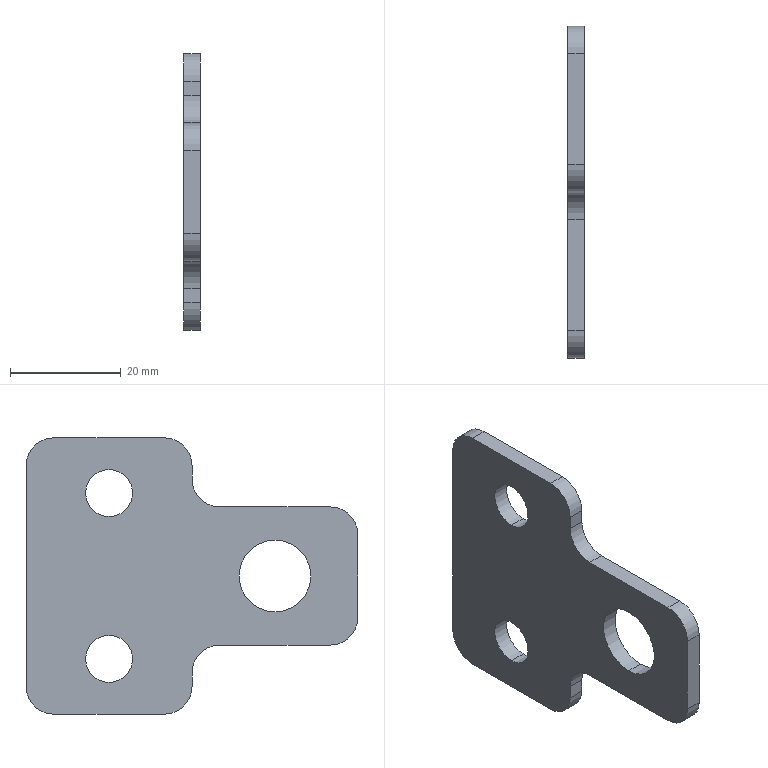Part | SolidWorks | features HoleWzd 2, Fillet 1, FlatPattern 1, ICE 1, SMBaseFlange 1, SheetMetal 1 | 1 solid | 24 faces | box 3 x 60 x 50 mm | volume 5947 mm3 | cylinder 14 | plane 10 | commonest cylinder face diameters 10 x8 8.5 x4 13 x2
STEP:
#1=CARTESIAN_POINT('',(-3.,-15.,6.5));
#2=VERTEX_POINT('',#1);
#3=CARTESIAN_POINT('',(-3.,-15.,-6.5));
#4=VERTEX_POINT('',#3);
#5=CARTESIAN_POINT('',(-3.,-15.,0.));
#6=DIRECTION('',(1.,0.,0.));
#7=DIRECTION('',(0.,0.,-1.));
#8=AXIS2_PLACEMENT_3D('',#5,#6,#7);
#9=CIRCLE('',#8,6.5);
#10=EDGE_CURVE('',#2,#4,#9,.T.);
#11=ORIENTED_EDGE('',*,*,#10,.F.);
#12=CARTESIAN_POINT('',(0.,-15.,6.5));
#13=VERTEX_POINT('',#12);
#14=CARTESIAN_POINT('',(0.,-15.,6.5));
#15=DIRECTION('',(1.,0.,0.));
#16=VECTOR('',#15,1000.);
#17=LINE('',#14,#16);
#18=EDGE_CURVE('',#2,#13,#17,.T.);
#19=ORIENTED_EDGE('',*,*,#18,.T.);
#20=CARTESIAN_POINT('',(0.,-15.,-6.5));
#21=VERTEX_POINT('',#20);
#22=CARTESIAN_POINT('',(0.,-15.,0.));
#23=DIRECTION('',(1.,0.,0.));
#24=DIRECTION('',(0.,0.,-1.));
#25=AXIS2_PLACEMENT_3D('',#22,#23,#24);
#26=CIRCLE('',#25,6.5);
#27=EDGE_CURVE('',#13,#21,#26,.T.);
#28=ORIENTED_EDGE('',*,*,#27,.T.);
#29=CARTESIAN_POINT('',(0.,-15.,-6.5));
#30=DIRECTION('',(1.,0.,0.));
#31=VECTOR('',#30,1000.);
#32=LINE('',#29,#31);
#33=EDGE_CURVE('',#4,#21,#32,.T.);
#34=ORIENTED_EDGE('',*,*,#33,.F.);
#35=EDGE_LOOP('',(#11,#19,#28,#34));
#36=FACE_OUTER_BOUND('',#35,.T.);
#37=CARTESIAN_POINT('',(0.,-15.,0.));
#38=DIRECTION('',(1.,0.,0.));
#39=DIRECTION('',(0.,0.,-1.));
#40=AXIS2_PLACEMENT_3D('',#37,#38,#39);
#41=CYLINDRICAL_SURFACE('',#40,6.5);
#42=ADVANCED_FACE('',(#36),#41,.F.);
#43=CARTESIAN_POINT('',(-3.,15.,19.25));
#44=VERTEX_POINT('',#43);
#45=CARTESIAN_POINT('',(-3.,15.,10.75));
#46=VERTEX_POINT('',#45);
#47=CARTESIAN_POINT('',(-3.,15.,15.));
#48=DIRECTION('',(1.,0.,0.));
#49=DIRECTION('',(0.,0.,-1.));
#50=AXIS2_PLACEMENT_3D('',#47,#48,#49);
#51=CIRCLE('',#50,4.25);
#52=EDGE_CURVE('',#44,#46,#51,.T.);
#53=ORIENTED_EDGE('',*,*,#52,.F.);
#54=CARTESIAN_POINT('',(0.,15.,19.25));
#55=VERTEX_POINT('',#54);
#56=CARTESIAN_POINT('',(0.,15.,19.25));
#57=DIRECTION('',(1.,0.,0.));
#58=VECTOR('',#57,1000.);
#59=LINE('',#56,#58);
#60=EDGE_CURVE('',#44,#55,#59,.T.);
#61=ORIENTED_EDGE('',*,*,#60,.T.);
#62=CARTESIAN_POINT('',(0.,15.,10.75));
#63=VERTEX_POINT('',#62);
#64=CARTESIAN_POINT('',(0.,15.,15.));
#65=DIRECTION('',(1.,0.,0.));
#66=DIRECTION('',(0.,0.,-1.));
#67=AXIS2_PLACEMENT_3D('',#64,#65,#66);
#68=CIRCLE('',#67,4.25);
#69=EDGE_CURVE('',#55,#63,#68,.T.);
#70=ORIENTED_EDGE('',*,*,#69,.T.);
#71=CARTESIAN_POINT('',(0.,15.,10.75));
#72=DIRECTION('',(1.,0.,0.));
#73=VECTOR('',#72,1000.);
#74=LINE('',#71,#73);
#75=EDGE_CURVE('',#46,#63,#74,.T.);
#76=ORIENTED_EDGE('',*,*,#75,.F.);
#77=EDGE_LOOP('',(#53,#61,#70,#76));
#78=FACE_OUTER_BOUND('',#77,.T.);
#79=CARTESIAN_POINT('',(0.,15.,15.));
#80=DIRECTION('',(1.,0.,0.));
#81=DIRECTION('',(0.,0.,-1.));
#82=AXIS2_PLACEMENT_3D('',#79,#80,#81);
#83=CYLINDRICAL_SURFACE('',#82,4.25);
#84=ADVANCED_FACE('',(#78),#83,.F.);
#85=CARTESIAN_POINT('',(-3.,15.,-10.75));
#86=VERTEX_POINT('',#85);
#87=CARTESIAN_POINT('',(-3.,15.,-19.25));
#88=VERTEX_POINT('',#87);
#89=CARTESIAN_POINT('',(-3.,15.,-15.));
#90=DIRECTION('',(1.,0.,0.));
#91=DIRECTION('',(0.,0.,-1.));
#92=AXIS2_PLACEMENT_3D('',#89,#90,#91);
#93=CIRCLE('',#92,4.25);
#94=EDGE_CURVE('',#86,#88,#93,.T.);
#95=ORIENTED_EDGE('',*,*,#94,.F.);
#96=CARTESIAN_POINT('',(0.,15.,-10.75));
#97=VERTEX_POINT('',#96);
#98=CARTESIAN_POINT('',(0.,15.,-10.75));
#99=DIRECTION('',(1.,0.,0.));
#100=VECTOR('',#99,1000.);
#101=LINE('',#98,#100);
#102=EDGE_CURVE('',#86,#97,#101,.T.);
#103=ORIENTED_EDGE('',*,*,#102,.T.);
#104=CARTESIAN_POINT('',(0.,15.,-19.25));
#105=VERTEX_POINT('',#104);
#106=CARTESIAN_POINT('',(0.,15.,-15.));
#107=DIRECTION('',(1.,0.,0.));
#108=DIRECTION('',(0.,0.,-1.));
#109=AXIS2_PLACEMENT_3D('',#106,#107,#108);
#110=CIRCLE('',#109,4.25);
#111=EDGE_CURVE('',#97,#105,#110,.T.);
#112=ORIENTED_EDGE('',*,*,#111,.T.);
#113=CARTESIAN_POINT('',(0.,15.,-19.25));
#114=DIRECTION('',(1.,0.,0.));
#115=VECTOR('',#114,1000.);
#116=LINE('',#113,#115);
#117=EDGE_CURVE('',#88,#105,#116,.T.);
#118=ORIENTED_EDGE('',*,*,#117,.F.);
#119=EDGE_LOOP('',(#95,#103,#112,#118));
#120=FACE_OUTER_BOUND('',#119,.T.);
#121=CARTESIAN_POINT('',(0.,15.,-15.));
#122=DIRECTION('',(1.,0.,0.));
#123=DIRECTION('',(0.,0.,-1.));
#124=AXIS2_PLACEMENT_3D('',#121,#122,#123);
#125=CYLINDRICAL_SURFACE('',#124,4.25);
#126=ADVANCED_FACE('',(#120),#125,.F.);
#127=CARTESIAN_POINT('',(0.,5.,-25.));
#128=VERTEX_POINT('',#127);
#129=CARTESIAN_POINT('',(0.,25.,-25.));
#130=VERTEX_POINT('',#129);
#131=CARTESIAN_POINT('',(0.,30.,-25.));
#132=DIRECTION('',(0.,1.,0.));
#133=VECTOR('',#132,1000.);
#134=LINE('',#131,#133);
#135=EDGE_CURVE('',#128,#130,#134,.T.);
#136=ORIENTED_EDGE('',*,*,#135,.F.);
#137=CARTESIAN_POINT('',(-3.,5.,-25.));
#138=VERTEX_POINT('',#137);
#139=CARTESIAN_POINT('',(-3.,5.,-25.));
#140=DIRECTION('',(-1.,0.,0.));
#141=VECTOR('',#140,1000.);
#142=LINE('',#139,#141);
#143=EDGE_CURVE('',#128,#138,#142,.T.);
#144=ORIENTED_EDGE('',*,*,#143,.T.);
#145=CARTESIAN_POINT('',(-3.,25.,-25.));
#146=VERTEX_POINT('',#145);
#147=CARTESIAN_POINT('',(-3.,30.,-25.));
#148=DIRECTION('',(0.,1.,0.));
#149=VECTOR('',#148,1000.);
#150=LINE('',#147,#149);
#151=EDGE_CURVE('',#138,#146,#150,.T.);
#152=ORIENTED_EDGE('',*,*,#151,.T.);
#153=CARTESIAN_POINT('',(-3.,25.,-25.));
#154=DIRECTION('',(1.,0.,0.));
#155=VECTOR('',#154,1000.);
#156=LINE('',#153,#155);
#157=EDGE_CURVE('',#146,#130,#156,.T.);
#158=ORIENTED_EDGE('',*,*,#157,.T.);
#159=EDGE_LOOP('',(#136,#144,#152,#158));
#160=FACE_OUTER_BOUND('',#159,.T.);
#161=CARTESIAN_POINT('',(-3.,30.,-25.));
#162=DIRECTION('',(0.,0.,-1.));
#163=DIRECTION('',(0.,1.,0.));
#164=AXIS2_PLACEMENT_3D('',#161,#162,#163);
#165=PLANE('',#164);
#166=ADVANCED_FACE('',(#160),#165,.T.);
#167=CARTESIAN_POINT('',(0.,-30.,7.5));
#168=VERTEX_POINT('',#167);
#169=CARTESIAN_POINT('',(0.,-30.,-7.5));
#170=VERTEX_POINT('',#169);
#171=CARTESIAN_POINT('',(0.,-30.,25.));
#172=DIRECTION('',(0.,0.,-1.));
#173=VECTOR('',#172,1000.);
#174=LINE('',#171,#173);
#175=EDGE_CURVE('',#168,#170,#174,.T.);
#176=ORIENTED_EDGE('',*,*,#175,.F.);
#177=CARTESIAN_POINT('',(-3.,-30.,7.5));
#178=VERTEX_POINT('',#177);
#179=CARTESIAN_POINT('',(-3.,-30.,7.5));
#180=DIRECTION('',(-1.,0.,0.));
#181=VECTOR('',#180,1000.);
#182=LINE('',#179,#181);
#183=EDGE_CURVE('',#168,#178,#182,.T.);
#184=ORIENTED_EDGE('',*,*,#183,.T.);
#185=CARTESIAN_POINT('',(-3.,-30.,-7.5));
#186=VERTEX_POINT('',#185);
#187=CARTESIAN_POINT('',(-3.,-30.,25.));
#188=DIRECTION('',(0.,0.,-1.));
#189=VECTOR('',#188,1000.);
#190=LINE('',#187,#189);
#191=EDGE_CURVE('',#178,#186,#190,.T.);
#192=ORIENTED_EDGE('',*,*,#191,.T.);
#193=CARTESIAN_POINT('',(0.,-30.,-7.5));
#194=DIRECTION('',(1.,0.,0.));
#195=VECTOR('',#194,1000.);
#196=LINE('',#193,#195);
#197=EDGE_CURVE('',#186,#170,#196,.T.);
#198=ORIENTED_EDGE('',*,*,#197,.T.);
#199=EDGE_LOOP('',(#176,#184,#192,#198));
#200=FACE_OUTER_BOUND('',#199,.T.);
#201=CARTESIAN_POINT('',(-3.,-30.,25.));
#202=DIRECTION('',(0.,-1.,0.));
#203=DIRECTION('',(0.,0.,-1.));
#204=AXIS2_PLACEMENT_3D('',#201,#202,#203);
#205=PLANE('',#204);
#206=ADVANCED_FACE('',(#200),#205,.T.);
#207=CARTESIAN_POINT('',(-3.,25.,25.));
#208=VERTEX_POINT('',#207);
#209=CARTESIAN_POINT('',(-3.,5.,25.));
#210=VERTEX_POINT('',#209);
#211=CARTESIAN_POINT('',(-3.,30.,25.));
#212=DIRECTION('',(0.,-1.,0.));
#213=VECTOR('',#212,1000.);
#214=LINE('',#211,#213);
#215=EDGE_CURVE('',#208,#210,#214,.T.);
#216=ORIENTED_EDGE('',*,*,#215,.T.);
#217=CARTESIAN_POINT('',(0.,5.,25.));
#218=VERTEX_POINT('',#217);
#219=CARTESIAN_POINT('',(0.,5.,25.));
#220=DIRECTION('',(1.,0.,0.));
#221=VECTOR('',#220,1000.);
#222=LINE('',#219,#221);
#223=EDGE_CURVE('',#210,#218,#222,.T.);
#224=ORIENTED_EDGE('',*,*,#223,.T.);
#225=CARTESIAN_POINT('',(0.,25.,25.));
#226=VERTEX_POINT('',#225);
#227=CARTESIAN_POINT('',(0.,30.,25.));
#228=DIRECTION('',(0.,-1.,0.));
#229=VECTOR('',#228,1000.);
#230=LINE('',#227,#229);
#231=EDGE_CURVE('',#226,#218,#230,.T.);
#232=ORIENTED_EDGE('',*,*,#231,.F.);
#233=CARTESIAN_POINT('',(-3.,25.,25.));
#234=DIRECTION('',(-1.,0.,0.));
#235=VECTOR('',#234,1000.);
#236=LINE('',#233,#235);
#237=EDGE_CURVE('',#226,#208,#236,.T.);
#238=ORIENTED_EDGE('',*,*,#237,.T.);
#239=EDGE_LOOP('',(#216,#224,#232,#238));
#240=FACE_OUTER_BOUND('',#239,.T.);
#241=CARTESIAN_POINT('',(-3.,30.,25.));
#242=DIRECTION('',(0.,0.,1.));
#243=DIRECTION('',(0.,-1.,0.));
#244=AXIS2_PLACEMENT_3D('',#241,#242,#243);
#245=PLANE('',#244);
#246=ADVANCED_FACE('',(#240),#245,.T.);
#247=CARTESIAN_POINT('',(0.,30.,-20.));
#248=VERTEX_POINT('',#247);
#249=CARTESIAN_POINT('',(0.,30.,20.));
#250=VERTEX_POINT('',#249);
#251=CARTESIAN_POINT('',(0.,30.,25.));
#252=DIRECTION('',(0.,0.,1.));
#253=VECTOR('',#252,1000.);
#254=LINE('',#251,#253);
#255=EDGE_CURVE('',#248,#250,#254,.T.);
#256=ORIENTED_EDGE('',*,*,#255,.F.);
#257=CARTESIAN_POINT('',(-3.,30.,-20.));
#258=VERTEX_POINT('',#257);
#259=CARTESIAN_POINT('',(-3.,30.,-20.));
#260=DIRECTION('',(-1.,0.,0.));
#261=VECTOR('',#260,1000.);
#262=LINE('',#259,#261);
#263=EDGE_CURVE('',#248,#258,#262,.T.);
#264=ORIENTED_EDGE('',*,*,#263,.T.);
#265=CARTESIAN_POINT('',(-3.,30.,20.));
#266=VERTEX_POINT('',#265);
#267=CARTESIAN_POINT('',(-3.,30.,25.));
#268=DIRECTION('',(0.,0.,1.));
#269=VECTOR('',#268,1000.);
#270=LINE('',#267,#269);
#271=EDGE_CURVE('',#258,#266,#270,.T.);
#272=ORIENTED_EDGE('',*,*,#271,.T.);
#273=CARTESIAN_POINT('',(-3.,30.,20.));
#274=DIRECTION('',(1.,0.,0.));
#275=VECTOR('',#274,1000.);
#276=LINE('',#273,#275);
#277=EDGE_CURVE('',#266,#250,#276,.T.);
#278=ORIENTED_EDGE('',*,*,#277,.T.);
#279=EDGE_LOOP('',(#256,#264,#272,#278));
#280=FACE_OUTER_BOUND('',#279,.T.);
#281=CARTESIAN_POINT('',(-3.,30.,25.));
#282=DIRECTION('',(0.,1.,0.));
#283=DIRECTION('',(0.,0.,1.));
#284=AXIS2_PLACEMENT_3D('',#281,#282,#283);
#285=PLANE('',#284);
#286=ADVANCED_FACE('',(#280),#285,.T.);
#287=CARTESIAN_POINT('',(-3.,-15.,0.));
#288=DIRECTION('',(1.,0.,0.));
#289=DIRECTION('',(0.,0.,-1.));
#290=AXIS2_PLACEMENT_3D('',#287,#288,#289);
#291=CIRCLE('',#290,6.5);
#292=EDGE_CURVE('',#4,#2,#291,.T.);
#293=ORIENTED_EDGE('',*,*,#292,.T.);
#294=ORIENTED_EDGE('',*,*,#10,.T.);
#295=EDGE_LOOP('',(#293,#294));
#296=FACE_BOUND('',#295,.T.);
#297=CARTESIAN_POINT('',(-3.,15.,15.));
#298=DIRECTION('',(1.,0.,0.));
#299=DIRECTION('',(0.,0.,-1.));
#300=AXIS2_PLACEMENT_3D('',#297,#298,#299);
#301=CIRCLE('',#300,4.25);
#302=EDGE_CURVE('',#46,#44,#301,.T.);
#303=ORIENTED_EDGE('',*,*,#302,.T.);
#304=ORIENTED_EDGE('',*,*,#52,.T.);
#305=EDGE_LOOP('',(#303,#304));
#306=FACE_BOUND('',#305,.T.);
#307=CARTESIAN_POINT('',(-3.,15.,-15.));
#308=DIRECTION('',(1.,0.,0.));
#309=DIRECTION('',(0.,0.,-1.));
#310=AXIS2_PLACEMENT_3D('',#307,#308,#309);
#311=CIRCLE('',#310,4.25);
#312=EDGE_CURVE('',#88,#86,#311,.T.);
#313=ORIENTED_EDGE('',*,*,#312,.T.);
#314=ORIENTED_EDGE('',*,*,#94,.T.);
#315=EDGE_LOOP('',(#313,#314));
#316=FACE_BOUND('',#315,.T.);
#317=ORIENTED_EDGE('',*,*,#191,.F.);
#318=CARTESIAN_POINT('',(-3.,-25.,12.5));
#319=VERTEX_POINT('',#318);
#320=CARTESIAN_POINT('',(-3.,-25.,7.5));
#321=DIRECTION('',(-1.,0.,0.));
#322=DIRECTION('',(0.,0.,-1.));
#323=AXIS2_PLACEMENT_3D('',#320,#321,#322);
#324=CIRCLE('',#323,5.);
#325=EDGE_CURVE('',#178,#319,#324,.T.);
#326=ORIENTED_EDGE('',*,*,#325,.T.);
#327=CARTESIAN_POINT('',(-3.,-5.,12.5));
#328=VERTEX_POINT('',#327);
#329=CARTESIAN_POINT('',(-3.,-30.,12.5));
#330=DIRECTION('',(0.,1.,0.));
#331=VECTOR('',#330,1000.);
#332=LINE('',#329,#331);
#333=EDGE_CURVE('',#319,#328,#332,.T.);
#334=ORIENTED_EDGE('',*,*,#333,.T.);
#335=CARTESIAN_POINT('',(-3.,0.,17.5));
#336=VERTEX_POINT('',#335);
#337=CARTESIAN_POINT('',(-3.,-5.,17.5));
#338=DIRECTION('',(1.,0.,0.));
#339=DIRECTION('',(0.,0.,-1.));
#340=AXIS2_PLACEMENT_3D('',#337,#338,#339);
#341=CIRCLE('',#340,5.);
#342=EDGE_CURVE('',#328,#336,#341,.T.);
#343=ORIENTED_EDGE('',*,*,#342,.T.);
#344=CARTESIAN_POINT('',(-3.,0.,20.));
#345=VERTEX_POINT('',#344);
#346=CARTESIAN_POINT('',(-3.,0.,25.));
#347=DIRECTION('',(0.,0.,1.));
#348=VECTOR('',#347,1000.);
#349=LINE('',#346,#348);
#350=EDGE_CURVE('',#336,#345,#349,.T.);
#351=ORIENTED_EDGE('',*,*,#350,.T.);
#352=CARTESIAN_POINT('',(-3.,5.,20.));
#353=DIRECTION('',(-1.,0.,0.));
#354=DIRECTION('',(0.,0.,-1.));
#355=AXIS2_PLACEMENT_3D('',#352,#353,#354);
#356=CIRCLE('',#355,5.);
#357=EDGE_CURVE('',#345,#210,#356,.T.);
#358=ORIENTED_EDGE('',*,*,#357,.T.);
#359=ORIENTED_EDGE('',*,*,#215,.F.);
#360=CARTESIAN_POINT('',(-3.,25.,20.));
#361=DIRECTION('',(-1.,0.,0.));
#362=DIRECTION('',(0.,0.,-1.));
#363=AXIS2_PLACEMENT_3D('',#360,#361,#362);
#364=CIRCLE('',#363,5.);
#365=EDGE_CURVE('',#208,#266,#364,.T.);
#366=ORIENTED_EDGE('',*,*,#365,.T.);
#367=ORIENTED_EDGE('',*,*,#271,.F.);
#368=CARTESIAN_POINT('',(-3.,25.,-20.));
#369=DIRECTION('',(-1.,0.,0.));
#370=DIRECTION('',(0.,0.,-1.));
#371=AXIS2_PLACEMENT_3D('',#368,#369,#370);
#372=CIRCLE('',#371,5.);
#373=EDGE_CURVE('',#258,#146,#372,.T.);
#374=ORIENTED_EDGE('',*,*,#373,.T.);
#375=ORIENTED_EDGE('',*,*,#151,.F.);
#376=CARTESIAN_POINT('',(-3.,0.,-20.));
#377=VERTEX_POINT('',#376);
#378=CARTESIAN_POINT('',(-3.,5.,-20.));
#379=DIRECTION('',(-1.,0.,0.));
#380=DIRECTION('',(0.,0.,-1.));
#381=AXIS2_PLACEMENT_3D('',#378,#379,#380);
#382=CIRCLE('',#381,5.);
#383=EDGE_CURVE('',#138,#377,#382,.T.);
#384=ORIENTED_EDGE('',*,*,#383,.T.);
#385=CARTESIAN_POINT('',(-3.,0.,-17.5));
#386=VERTEX_POINT('',#385);
#387=CARTESIAN_POINT('',(-3.,0.,-25.));
#388=DIRECTION('',(0.,0.,1.));
#389=VECTOR('',#388,1000.);
#390=LINE('',#387,#389);
#391=EDGE_CURVE('',#377,#386,#390,.T.);
#392=ORIENTED_EDGE('',*,*,#391,.T.);
#393=CARTESIAN_POINT('',(-3.,-5.,-12.5));
#394=VERTEX_POINT('',#393);
#395=CARTESIAN_POINT('',(-3.,-5.,-17.5));
#396=DIRECTION('',(1.,0.,0.));
#397=DIRECTION('',(0.,0.,-1.));
#398=AXIS2_PLACEMENT_3D('',#395,#396,#397);
#399=CIRCLE('',#398,5.);
#400=EDGE_CURVE('',#386,#394,#399,.T.);
#401=ORIENTED_EDGE('',*,*,#400,.T.);
#402=CARTESIAN_POINT('',(-3.,-25.,-12.5));
#403=VERTEX_POINT('',#402);
#404=CARTESIAN_POINT('',(-3.,-30.,-12.5));
#405=DIRECTION('',(0.,-1.,0.));
#406=VECTOR('',#405,1000.);
#407=LINE('',#404,#406);
#408=EDGE_CURVE('',#394,#403,#407,.T.);
#409=ORIENTED_EDGE('',*,*,#408,.T.);
#410=CARTESIAN_POINT('',(-3.,-25.,-7.5));
#411=DIRECTION('',(-1.,0.,0.));
#412=DIRECTION('',(0.,0.,-1.));
#413=AXIS2_PLACEMENT_3D('',#410,#411,#412);
#414=CIRCLE('',#413,5.);
#415=EDGE_CURVE('',#403,#186,#414,.T.);
#416=ORIENTED_EDGE('',*,*,#415,.T.);
#417=EDGE_LOOP('',(#317,#326,#334,#343,#351,#358,#359,#366,#367,#374,#375,#384,#392,#401,#409,#416));
#418=FACE_OUTER_BOUND('',#417,.T.);
#419=CARTESIAN_POINT('',(-3.,0.,0.));
#420=DIRECTION('',(1.,0.,0.));
#421=DIRECTION('',(0.,0.,-1.));
#422=AXIS2_PLACEMENT_3D('',#419,#420,#421);
#423=PLANE('',#422);
#424=ADVANCED_FACE('',(#296,#306,#316,#418),#423,.F.);
#425=CARTESIAN_POINT('',(0.,-15.,0.));
#426=DIRECTION('',(1.,0.,0.));
#427=DIRECTION('',(0.,0.,-1.));
#428=AXIS2_PLACEMENT_3D('',#425,#426,#427);
#429=CIRCLE('',#428,6.5);
#430=EDGE_CURVE('',#21,#13,#429,.T.);
#431=ORIENTED_EDGE('',*,*,#430,.F.);
#432=ORIENTED_EDGE('',*,*,#27,.F.);
#433=EDGE_LOOP('',(#431,#432));
#434=FACE_BOUND('',#433,.T.);
#435=CARTESIAN_POINT('',(0.,15.,15.));
#436=DIRECTION('',(1.,0.,0.));
#437=DIRECTION('',(0.,0.,-1.));
#438=AXIS2_PLACEMENT_3D('',#435,#436,#437);
#439=CIRCLE('',#438,4.25);
#440=EDGE_CURVE('',#63,#55,#439,.T.);
#441=ORIENTED_EDGE('',*,*,#440,.F.);
#442=ORIENTED_EDGE('',*,*,#69,.F.);
#443=EDGE_LOOP('',(#441,#442));
#444=FACE_BOUND('',#443,.T.);
#445=CARTESIAN_POINT('',(0.,15.,-15.));
#446=DIRECTION('',(1.,0.,0.));
#447=DIRECTION('',(0.,0.,-1.));
#448=AXIS2_PLACEMENT_3D('',#445,#446,#447);
#449=CIRCLE('',#448,4.25);
#450=EDGE_CURVE('',#105,#97,#449,.T.);
#451=ORIENTED_EDGE('',*,*,#450,.F.);
#452=ORIENTED_EDGE('',*,*,#111,.F.);
#453=EDGE_LOOP('',(#451,#452));
#454=FACE_BOUND('',#453,.T.);
#455=CARTESIAN_POINT('',(0.,-25.,12.5));
#456=VERTEX_POINT('',#455);
#457=CARTESIAN_POINT('',(0.,-5.,12.5));
#458=VERTEX_POINT('',#457);
#459=CARTESIAN_POINT('',(0.,-30.,12.5));
#460=DIRECTION('',(0.,1.,0.));
#461=VECTOR('',#460,1000.);
#462=LINE('',#459,#461);
#463=EDGE_CURVE('',#456,#458,#462,.T.);
#464=ORIENTED_EDGE('',*,*,#463,.F.);
#465=CARTESIAN_POINT('',(0.,-25.,7.5));
#466=DIRECTION('',(1.,0.,0.));
#467=DIRECTION('',(0.,0.,-1.));
#468=AXIS2_PLACEMENT_3D('',#465,#466,#467);
#469=CIRCLE('',#468,5.);
#470=EDGE_CURVE('',#456,#168,#469,.T.);
#471=ORIENTED_EDGE('',*,*,#470,.T.);
#472=ORIENTED_EDGE('',*,*,#175,.T.);
#473=CARTESIAN_POINT('',(0.,-25.,-12.5));
#474=VERTEX_POINT('',#473);
#475=CARTESIAN_POINT('',(0.,-25.,-7.5));
#476=DIRECTION('',(1.,0.,0.));
#477=DIRECTION('',(0.,0.,-1.));
#478=AXIS2_PLACEMENT_3D('',#475,#476,#477);
#479=CIRCLE('',#478,5.);
#480=EDGE_CURVE('',#170,#474,#479,.T.);
#481=ORIENTED_EDGE('',*,*,#480,.T.);
#482=CARTESIAN_POINT('',(0.,-5.,-12.5));
#483=VERTEX_POINT('',#482);
#484=CARTESIAN_POINT('',(0.,-30.,-12.5));
#485=DIRECTION('',(0.,-1.,0.));
#486=VECTOR('',#485,1000.);
#487=LINE('',#484,#486);
#488=EDGE_CURVE('',#483,#474,#487,.T.);
#489=ORIENTED_EDGE('',*,*,#488,.F.);
#490=CARTESIAN_POINT('',(0.,0.,-17.5));
#491=VERTEX_POINT('',#490);
#492=CARTESIAN_POINT('',(0.,-5.,-17.5));
#493=DIRECTION('',(-1.,0.,0.));
#494=DIRECTION('',(0.,0.,-1.));
#495=AXIS2_PLACEMENT_3D('',#492,#493,#494);
#496=CIRCLE('',#495,5.);
#497=EDGE_CURVE('',#483,#491,#496,.T.);
#498=ORIENTED_EDGE('',*,*,#497,.T.);
#499=CARTESIAN_POINT('',(0.,0.,-20.));
#500=VERTEX_POINT('',#499);
#501=CARTESIAN_POINT('',(0.,0.,-25.));
#502=DIRECTION('',(0.,0.,1.));
#503=VECTOR('',#502,1000.);
#504=LINE('',#501,#503);
#505=EDGE_CURVE('',#500,#491,#504,.T.);
#506=ORIENTED_EDGE('',*,*,#505,.F.);
#507=CARTESIAN_POINT('',(0.,5.,-20.));
#508=DIRECTION('',(1.,0.,0.));
#509=DIRECTION('',(0.,0.,-1.));
#510=AXIS2_PLACEMENT_3D('',#507,#508,#509);
#511=CIRCLE('',#510,5.);
#512=EDGE_CURVE('',#500,#128,#511,.T.);
#513=ORIENTED_EDGE('',*,*,#512,.T.);
#514=ORIENTED_EDGE('',*,*,#135,.T.);
#515=CARTESIAN_POINT('',(0.,25.,-20.));
#516=DIRECTION('',(1.,0.,0.));
#517=DIRECTION('',(0.,0.,-1.));
#518=AXIS2_PLACEMENT_3D('',#515,#516,#517);
#519=CIRCLE('',#518,5.);
#520=EDGE_CURVE('',#130,#248,#519,.T.);
#521=ORIENTED_EDGE('',*,*,#520,.T.);
#522=ORIENTED_EDGE('',*,*,#255,.T.);
#523=CARTESIAN_POINT('',(0.,25.,20.));
#524=DIRECTION('',(1.,0.,0.));
#525=DIRECTION('',(0.,0.,-1.));
#526=AXIS2_PLACEMENT_3D('',#523,#524,#525);
#527=CIRCLE('',#526,5.);
#528=EDGE_CURVE('',#250,#226,#527,.T.);
#529=ORIENTED_EDGE('',*,*,#528,.T.);
#530=ORIENTED_EDGE('',*,*,#231,.T.);
#531=CARTESIAN_POINT('',(0.,0.,20.));
#532=VERTEX_POINT('',#531);
#533=CARTESIAN_POINT('',(0.,5.,20.));
#534=DIRECTION('',(1.,0.,0.));
#535=DIRECTION('',(0.,0.,-1.));
#536=AXIS2_PLACEMENT_3D('',#533,#534,#535);
#537=CIRCLE('',#536,5.);
#538=EDGE_CURVE('',#218,#532,#537,.T.);
#539=ORIENTED_EDGE('',*,*,#538,.T.);
#540=CARTESIAN_POINT('',(0.,0.,17.5));
#541=VERTEX_POINT('',#540);
#542=CARTESIAN_POINT('',(0.,0.,25.));
#543=DIRECTION('',(0.,0.,1.));
#544=VECTOR('',#543,1000.);
#545=LINE('',#542,#544);
#546=EDGE_CURVE('',#541,#532,#545,.T.);
#547=ORIENTED_EDGE('',*,*,#546,.F.);
#548=CARTESIAN_POINT('',(0.,-5.,17.5));
#549=DIRECTION('',(-1.,0.,0.));
#550=DIRECTION('',(0.,0.,-1.));
#551=AXIS2_PLACEMENT_3D('',#548,#549,#550);
#552=CIRCLE('',#551,5.);
#553=EDGE_CURVE('',#541,#458,#552,.T.);
#554=ORIENTED_EDGE('',*,*,#553,.T.);
#555=EDGE_LOOP('',(#464,#471,#472,#481,#489,#498,#506,#513,#514,#521,#522,#529,#530,#539,#547,#554));
#556=FACE_OUTER_BOUND('',#555,.T.);
#557=CARTESIAN_POINT('',(0.,0.,0.));
#558=DIRECTION('',(1.,0.,0.));
#559=DIRECTION('',(0.,0.,-1.));
#560=AXIS2_PLACEMENT_3D('',#557,#558,#559);
#561=PLANE('',#560);
#562=ADVANCED_FACE('',(#434,#444,#454,#556),#561,.T.);
#563=ORIENTED_EDGE('',*,*,#350,.F.);
#564=CARTESIAN_POINT('',(0.,0.,17.5));
#565=DIRECTION('',(1.,0.,0.));
#566=VECTOR('',#565,1000.);
#567=LINE('',#564,#566);
#568=EDGE_CURVE('',#336,#541,#567,.T.);
#569=ORIENTED_EDGE('',*,*,#568,.T.);
#570=ORIENTED_EDGE('',*,*,#546,.T.);
#571=CARTESIAN_POINT('',(-3.,0.,20.));
#572=DIRECTION('',(-1.,0.,0.));
#573=VECTOR('',#572,1000.);
#574=LINE('',#571,#573);
#575=EDGE_CURVE('',#532,#345,#574,.T.);
#576=ORIENTED_EDGE('',*,*,#575,.T.);
#577=EDGE_LOOP('',(#563,#569,#570,#576));
#578=FACE_OUTER_BOUND('',#577,.T.);
#579=CARTESIAN_POINT('',(-3.,0.,25.));
#580=DIRECTION('',(0.,1.,0.));
#581=DIRECTION('',(0.,0.,1.));
#582=AXIS2_PLACEMENT_3D('',#579,#580,#581);
#583=PLANE('',#582);
#584=ADVANCED_FACE('',(#578),#583,.F.);
#585=ORIENTED_EDGE('',*,*,#333,.F.);
#586=CARTESIAN_POINT('',(0.,-25.,12.5));
#587=DIRECTION('',(1.,0.,0.));
#588=VECTOR('',#587,1000.);
#589=LINE('',#586,#588);
#590=EDGE_CURVE('',#319,#456,#589,.T.);
#591=ORIENTED_EDGE('',*,*,#590,.T.);
#592=ORIENTED_EDGE('',*,*,#463,.T.);
#593=CARTESIAN_POINT('',(-3.,-5.,12.5));
#594=DIRECTION('',(-1.,0.,0.));
#595=VECTOR('',#594,1000.);
#596=LINE('',#593,#595);
#597=EDGE_CURVE('',#458,#328,#596,.T.);
#598=ORIENTED_EDGE('',*,*,#597,.T.);
#599=EDGE_LOOP('',(#585,#591,#592,#598));
#600=FACE_OUTER_BOUND('',#599,.T.);
#601=CARTESIAN_POINT('',(-3.,-30.,12.5));
#602=DIRECTION('',(0.,0.,-1.));
#603=DIRECTION('',(-1.,0.,0.));
#604=AXIS2_PLACEMENT_3D('',#601,#602,#603);
#605=PLANE('',#604);
#606=ADVANCED_FACE('',(#600),#605,.F.);
#607=ORIENTED_EDGE('',*,*,#488,.T.);
#608=CARTESIAN_POINT('',(-3.,-25.,-12.5));
#609=DIRECTION('',(-1.,0.,0.));
#610=VECTOR('',#609,1000.);
#611=LINE('',#608,#610);
#612=EDGE_CURVE('',#474,#403,#611,.T.);
#613=ORIENTED_EDGE('',*,*,#612,.T.);
#614=ORIENTED_EDGE('',*,*,#408,.F.);
#615=CARTESIAN_POINT('',(0.,-5.,-12.5));
#616=DIRECTION('',(1.,0.,0.));
#617=VECTOR('',#616,1000.);
#618=LINE('',#615,#617);
#619=EDGE_CURVE('',#394,#483,#618,.T.);
#620=ORIENTED_EDGE('',*,*,#619,.T.);
#621=EDGE_LOOP('',(#607,#613,#614,#620));
#622=FACE_OUTER_BOUND('',#621,.T.);
#623=CARTESIAN_POINT('',(-3.,-30.,-12.5));
#624=DIRECTION('',(0.,0.,1.));
#625=DIRECTION('',(1.,0.,0.));
#626=AXIS2_PLACEMENT_3D('',#623,#624,#625);
#627=PLANE('',#626);
#628=ADVANCED_FACE('',(#622),#627,.F.);
#629=ORIENTED_EDGE('',*,*,#505,.T.);
#630=CARTESIAN_POINT('',(-3.,0.,-17.5));
#631=DIRECTION('',(-1.,0.,0.));
#632=VECTOR('',#631,1000.);
#633=LINE('',#630,#632);
#634=EDGE_CURVE('',#491,#386,#633,.T.);
#635=ORIENTED_EDGE('',*,*,#634,.T.);
#636=ORIENTED_EDGE('',*,*,#391,.F.);
#637=CARTESIAN_POINT('',(0.,0.,-20.));
#638=DIRECTION('',(1.,0.,0.));
#639=VECTOR('',#638,1000.);
#640=LINE('',#637,#639);
#641=EDGE_CURVE('',#377,#500,#640,.T.);
#642=ORIENTED_EDGE('',*,*,#641,.T.);
#643=EDGE_LOOP('',(#629,#635,#636,#642));
#644=FACE_OUTER_BOUND('',#643,.T.);
#645=CARTESIAN_POINT('',(-3.,0.,-25.));
#646=DIRECTION('',(0.,1.,0.));
#647=DIRECTION('',(0.,0.,1.));
#648=AXIS2_PLACEMENT_3D('',#645,#646,#647);
#649=PLANE('',#648);
#650=ADVANCED_FACE('',(#644),#649,.F.);
#651=ORIENTED_EDGE('',*,*,#102,.F.);
#652=ORIENTED_EDGE('',*,*,#312,.F.);
#653=ORIENTED_EDGE('',*,*,#117,.T.);
#654=ORIENTED_EDGE('',*,*,#450,.T.);
#655=EDGE_LOOP('',(#651,#652,#653,#654));
#656=FACE_OUTER_BOUND('',#655,.T.);
#657=CARTESIAN_POINT('',(0.,15.,-15.));
#658=DIRECTION('',(1.,0.,0.));
#659=DIRECTION('',(0.,0.,-1.));
#660=AXIS2_PLACEMENT_3D('',#657,#658,#659);
#661=CYLINDRICAL_SURFACE('',#660,4.25);
#662=ADVANCED_FACE('',(#656),#661,.F.);
#663=ORIENTED_EDGE('',*,*,#60,.F.);
#664=ORIENTED_EDGE('',*,*,#302,.F.);
#665=ORIENTED_EDGE('',*,*,#75,.T.);
#666=ORIENTED_EDGE('',*,*,#440,.T.);
#667=EDGE_LOOP('',(#663,#664,#665,#666));
#668=FACE_OUTER_BOUND('',#667,.T.);
#669=CARTESIAN_POINT('',(0.,15.,15.));
#670=DIRECTION('',(1.,0.,0.));
#671=DIRECTION('',(0.,0.,-1.));
#672=AXIS2_PLACEMENT_3D('',#669,#670,#671);
#673=CYLINDRICAL_SURFACE('',#672,4.25);
#674=ADVANCED_FACE('',(#668),#673,.F.);
#675=ORIENTED_EDGE('',*,*,#18,.F.);
#676=ORIENTED_EDGE('',*,*,#292,.F.);
#677=ORIENTED_EDGE('',*,*,#33,.T.);
#678=ORIENTED_EDGE('',*,*,#430,.T.);
#679=EDGE_LOOP('',(#675,#676,#677,#678));
#680=FACE_OUTER_BOUND('',#679,.T.);
#681=CARTESIAN_POINT('',(0.,-15.,0.));
#682=DIRECTION('',(1.,0.,0.));
#683=DIRECTION('',(0.,0.,-1.));
#684=AXIS2_PLACEMENT_3D('',#681,#682,#683);
#685=CYLINDRICAL_SURFACE('',#684,6.5);
#686=ADVANCED_FACE('',(#680),#685,.F.);
#687=ORIENTED_EDGE('',*,*,#325,.F.);
#688=ORIENTED_EDGE('',*,*,#183,.F.);
#689=ORIENTED_EDGE('',*,*,#470,.F.);
#690=ORIENTED_EDGE('',*,*,#590,.F.);
#691=EDGE_LOOP('',(#687,#688,#689,#690));
#692=FACE_OUTER_BOUND('',#691,.T.);
#693=CARTESIAN_POINT('',(-3.,-25.,7.5));
#694=DIRECTION('',(-1.,0.,0.));
#695=DIRECTION('',(0.,0.,1.));
#696=AXIS2_PLACEMENT_3D('',#693,#694,#695);
#697=CYLINDRICAL_SURFACE('',#696,5.);
#698=ADVANCED_FACE('',(#692),#697,.T.);
#699=ORIENTED_EDGE('',*,*,#415,.F.);
#700=ORIENTED_EDGE('',*,*,#612,.F.);
#701=ORIENTED_EDGE('',*,*,#480,.F.);
#702=ORIENTED_EDGE('',*,*,#197,.F.);
#703=EDGE_LOOP('',(#699,#700,#701,#702));
#704=FACE_OUTER_BOUND('',#703,.T.);
#705=CARTESIAN_POINT('',(-3.,-25.,-7.5));
#706=DIRECTION('',(-1.,0.,0.));
#707=DIRECTION('',(0.,0.,1.));
#708=AXIS2_PLACEMENT_3D('',#705,#706,#707);
#709=CYLINDRICAL_SURFACE('',#708,5.);
#710=ADVANCED_FACE('',(#704),#709,.T.);
#711=ORIENTED_EDGE('',*,*,#400,.F.);
#712=ORIENTED_EDGE('',*,*,#634,.F.);
#713=ORIENTED_EDGE('',*,*,#497,.F.);
#714=ORIENTED_EDGE('',*,*,#619,.F.);
#715=EDGE_LOOP('',(#711,#712,#713,#714));
#716=FACE_OUTER_BOUND('',#715,.T.);
#717=CARTESIAN_POINT('',(-3.,-5.,-17.5));
#718=DIRECTION('',(-1.,0.,0.));
#719=DIRECTION('',(0.,0.,1.));
#720=AXIS2_PLACEMENT_3D('',#717,#718,#719);
#721=CYLINDRICAL_SURFACE('',#720,5.);
#722=ADVANCED_FACE('',(#716),#721,.F.);
#723=ORIENTED_EDGE('',*,*,#383,.F.);
#724=ORIENTED_EDGE('',*,*,#143,.F.);
#725=ORIENTED_EDGE('',*,*,#512,.F.);
#726=ORIENTED_EDGE('',*,*,#641,.F.);
#727=EDGE_LOOP('',(#723,#724,#725,#726));
#728=FACE_OUTER_BOUND('',#727,.T.);
#729=CARTESIAN_POINT('',(-3.,5.,-20.));
#730=DIRECTION('',(-1.,0.,0.));
#731=DIRECTION('',(0.,0.,1.));
#732=AXIS2_PLACEMENT_3D('',#729,#730,#731);
#733=CYLINDRICAL_SURFACE('',#732,5.);
#734=ADVANCED_FACE('',(#728),#733,.T.);
#735=ORIENTED_EDGE('',*,*,#373,.F.);
#736=ORIENTED_EDGE('',*,*,#263,.F.);
#737=ORIENTED_EDGE('',*,*,#520,.F.);
#738=ORIENTED_EDGE('',*,*,#157,.F.);
#739=EDGE_LOOP('',(#735,#736,#737,#738));
#740=FACE_OUTER_BOUND('',#739,.T.);
#741=CARTESIAN_POINT('',(-3.,25.,-20.));
#742=DIRECTION('',(1.,0.,0.));
#743=DIRECTION('',(0.,0.,-1.));
#744=AXIS2_PLACEMENT_3D('',#741,#742,#743);
#745=CYLINDRICAL_SURFACE('',#744,5.);
#746=ADVANCED_FACE('',(#740),#745,.T.);
#747=ORIENTED_EDGE('',*,*,#342,.F.);
#748=ORIENTED_EDGE('',*,*,#597,.F.);
#749=ORIENTED_EDGE('',*,*,#553,.F.);
#750=ORIENTED_EDGE('',*,*,#568,.F.);
#751=EDGE_LOOP('',(#747,#748,#749,#750));
#752=FACE_OUTER_BOUND('',#751,.T.);
#753=CARTESIAN_POINT('',(-3.,-5.,17.5));
#754=DIRECTION('',(-1.,0.,0.));
#755=DIRECTION('',(0.,0.,1.));
#756=AXIS2_PLACEMENT_3D('',#753,#754,#755);
#757=CYLINDRICAL_SURFACE('',#756,5.);
#758=ADVANCED_FACE('',(#752),#757,.F.);
#759=ORIENTED_EDGE('',*,*,#357,.F.);
#760=ORIENTED_EDGE('',*,*,#575,.F.);
#761=ORIENTED_EDGE('',*,*,#538,.F.);
#762=ORIENTED_EDGE('',*,*,#223,.F.);
#763=EDGE_LOOP('',(#759,#760,#761,#762));
#764=FACE_OUTER_BOUND('',#763,.T.);
#765=CARTESIAN_POINT('',(-3.,5.,20.));
#766=DIRECTION('',(-1.,0.,0.));
#767=DIRECTION('',(0.,0.,1.));
#768=AXIS2_PLACEMENT_3D('',#765,#766,#767);
#769=CYLINDRICAL_SURFACE('',#768,5.);
#770=ADVANCED_FACE('',(#764),#769,.T.);
#771=ORIENTED_EDGE('',*,*,#365,.F.);
#772=ORIENTED_EDGE('',*,*,#237,.F.);
#773=ORIENTED_EDGE('',*,*,#528,.F.);
#774=ORIENTED_EDGE('',*,*,#277,.F.);
#775=EDGE_LOOP('',(#771,#772,#773,#774));
#776=FACE_OUTER_BOUND('',#775,.T.);
#777=CARTESIAN_POINT('',(-3.,25.,20.));
#778=DIRECTION('',(1.,0.,0.));
#779=DIRECTION('',(0.,0.,-1.));
#780=AXIS2_PLACEMENT_3D('',#777,#778,#779);
#781=CYLINDRICAL_SURFACE('',#780,5.);
#782=ADVANCED_FACE('',(#776),#781,.T.);
#783=CLOSED_SHELL('',(#42,#84,#126,#166,#206,#246,#286,#424,#562,#584,#606,#628,#650,#662,#674,#686,#698,#710,#722,#734,#746,#758,#770,#782));
#784=MANIFOLD_SOLID_BREP('',#783);
#785=CARTESIAN_POINT('',(0.,0.,0.));
#786=DIRECTION('',(0.,0.,1.));
#787=DIRECTION('',(1.,0.,0.));
#788=AXIS2_PLACEMENT_3D('',#785,#786,#787);
#789=(LENGTH_UNIT()NAMED_UNIT(*)SI_UNIT(.MILLI.,.METRE.));
#790=UNCERTAINTY_MEASURE_WITH_UNIT(LENGTH_MEASURE(0.00001),#789,'','');
#791=(NAMED_UNIT(*)PLANE_ANGLE_UNIT()SI_UNIT($,.RADIAN.));
#792=(NAMED_UNIT(*)SI_UNIT($,.STERADIAN.)SOLID_ANGLE_UNIT());
#793=(GEOMETRIC_REPRESENTATION_CONTEXT(3)GLOBAL_UNCERTAINTY_ASSIGNED_CONTEXT((#790))GLOBAL_UNIT_ASSIGNED_CONTEXT((#789,#791,#792))REPRESENTATION_CONTEXT('',''));
#794=ADVANCED_BREP_SHAPE_REPRESENTATION('',(#784,#788),#793);